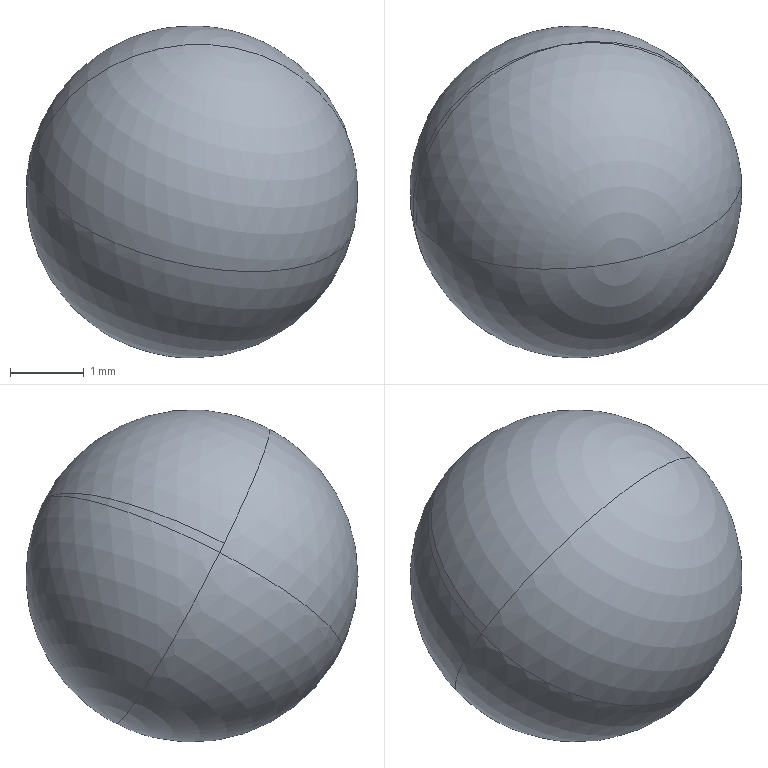Part | SolidWorks | features BaseBody 1 | 1 solid | 6 faces | box 4.5 x 4.5 x 4.5 mm | volume 47.713 mm3 | sphere 6
STEP:
#1=CARTESIAN_POINT('',(1921.673,-161.637,842.253));
#2=VERTEX_POINT('',#1);
#3=CARTESIAN_POINT('',(1924.058,-163.253,840.902));
#4=VERTEX_POINT('',#3);
#5=CARTESIAN_POINT('',(1921.862,-163.627,841.221));
#6=DIRECTION('',(-0.2015,0.436,-0.8771));
#7=DIRECTION('',(-0.08415,0.8844,0.459));
#8=AXIS2_PLACEMENT_3D('',#5,#6,#7);
#9=CIRCLE('',#8,2.25);
#10=EDGE_CURVE('',#2,#4,#9,.T.);
#11=ORIENTED_EDGE('',*,*,#10,.F.);
#12=CARTESIAN_POINT('',(1919.699,-164.062,841.662));
#13=VERTEX_POINT('',#12);
#14=CARTESIAN_POINT('',(1921.862,-163.627,841.221));
#15=DIRECTION('',(0.2623,-0.4247,0.8665));
#16=DIRECTION('',(0.,-0.8979,-0.4401));
#17=AXIS2_PLACEMENT_3D('',#14,#15,#16);
#18=CIRCLE('',#17,2.25);
#19=EDGE_CURVE('',#2,#13,#18,.T.);
#20=ORIENTED_EDGE('',*,*,#19,.T.);
#21=CARTESIAN_POINT('',(1921.862,-163.627,841.221));
#22=DIRECTION('',(-0.08415,0.8844,0.459));
#23=DIRECTION('',(0.2015,-0.436,0.8771));
#24=AXIS2_PLACEMENT_3D('',#21,#22,#23);
#25=CIRCLE('',#24,2.25);
#26=EDGE_CURVE('',#13,#4,#25,.T.);
#27=ORIENTED_EDGE('',*,*,#26,.T.);
#28=EDGE_LOOP('',(#11,#20,#27));
#29=FACE_OUTER_BOUND('',#28,.T.);
#30=CARTESIAN_POINT('',(1921.862,-163.627,841.221));
#31=DIRECTION('',(-0.2623,0.4247,-0.8665));
#32=DIRECTION('',(-0.9613,-0.1933,0.1963));
#33=AXIS2_PLACEMENT_3D('',#30,#31,#32);
#34=SPHERICAL_SURFACE('',#33,2.25);
#35=ADVANCED_FACE('',(#29),#34,.T.);
#36=CARTESIAN_POINT('',(1919.666,-164.001,841.539));
#37=VERTEX_POINT('',#36);
#38=CARTESIAN_POINT('',(1921.862,-163.627,841.221));
#39=DIRECTION('',(-0.2015,0.436,-0.8771));
#40=DIRECTION('',(-0.08415,0.8844,0.459));
#41=AXIS2_PLACEMENT_3D('',#38,#39,#40);
#42=CIRCLE('',#41,2.25);
#43=EDGE_CURVE('',#37,#2,#42,.T.);
#44=ORIENTED_EDGE('',*,*,#43,.T.);
#45=CARTESIAN_POINT('',(1924.025,-163.192,840.779));
#46=VERTEX_POINT('',#45);
#47=CARTESIAN_POINT('',(1921.862,-163.627,841.221));
#48=DIRECTION('',(-0.2623,0.4247,-0.8665));
#49=DIRECTION('',(0.,0.8979,0.4401));
#50=AXIS2_PLACEMENT_3D('',#47,#48,#49);
#51=CIRCLE('',#50,2.25);
#52=EDGE_CURVE('',#2,#46,#51,.T.);
#53=ORIENTED_EDGE('',*,*,#52,.T.);
#54=CARTESIAN_POINT('',(1921.862,-163.627,841.221));
#55=DIRECTION('',(0.08415,-0.8844,-0.459));
#56=DIRECTION('',(0.9759,0.1663,-0.1415));
#57=AXIS2_PLACEMENT_3D('',#54,#55,#56);
#58=CIRCLE('',#57,2.25);
#59=EDGE_CURVE('',#37,#46,#58,.T.);
#60=ORIENTED_EDGE('',*,*,#59,.F.);
#61=EDGE_LOOP('',(#44,#53,#60));
#62=FACE_OUTER_BOUND('',#61,.T.);
#63=CARTESIAN_POINT('',(1921.862,-163.627,841.221));
#64=DIRECTION('',(0.2623,-0.4247,0.8665));
#65=DIRECTION('',(0.9613,0.1933,-0.1963));
#66=AXIS2_PLACEMENT_3D('',#63,#64,#65);
#67=SPHERICAL_SURFACE('',#66,2.25);
#68=ADVANCED_FACE('',(#62),#67,.T.);
#69=ORIENTED_EDGE('',*,*,#59,.T.);
#70=CARTESIAN_POINT('',(1921.862,-163.627,841.221));
#71=DIRECTION('',(0.08415,-0.8844,-0.459));
#72=DIRECTION('',(0.9759,0.1663,-0.1415));
#73=AXIS2_PLACEMENT_3D('',#70,#71,#72);
#74=CIRCLE('',#73,2.25);
#75=EDGE_CURVE('',#46,#4,#74,.T.);
#76=ORIENTED_EDGE('',*,*,#75,.T.);
#77=CARTESIAN_POINT('',(1921.862,-163.627,841.221));
#78=DIRECTION('',(0.2015,-0.436,0.8771));
#79=DIRECTION('',(-0.9759,-0.1663,0.1415));
#80=AXIS2_PLACEMENT_3D('',#77,#78,#79);
#81=CIRCLE('',#80,2.25);
#82=EDGE_CURVE('',#37,#4,#81,.T.);
#83=ORIENTED_EDGE('',*,*,#82,.F.);
#84=EDGE_LOOP('',(#69,#76,#83));
#85=FACE_OUTER_BOUND('',#84,.T.);
#86=CARTESIAN_POINT('',(1921.862,-163.627,841.221));
#87=DIRECTION('',(-0.2623,0.4247,-0.8665));
#88=DIRECTION('',(-0.9613,-0.1933,0.1963));
#89=AXIS2_PLACEMENT_3D('',#86,#87,#88);
#90=SPHERICAL_SURFACE('',#89,2.25);
#91=ADVANCED_FACE('',(#85),#90,.T.);
#92=ORIENTED_EDGE('',*,*,#52,.F.);
#93=ORIENTED_EDGE('',*,*,#10,.T.);
#94=ORIENTED_EDGE('',*,*,#75,.F.);
#95=EDGE_LOOP('',(#92,#93,#94));
#96=FACE_OUTER_BOUND('',#95,.T.);
#97=CARTESIAN_POINT('',(1921.862,-163.627,841.221));
#98=DIRECTION('',(0.2623,-0.4247,0.8665));
#99=DIRECTION('',(0.9613,0.1933,-0.1963));
#100=AXIS2_PLACEMENT_3D('',#97,#98,#99);
#101=SPHERICAL_SURFACE('',#100,2.25);
#102=ADVANCED_FACE('',(#96),#101,.T.);
#103=ORIENTED_EDGE('',*,*,#19,.F.);
#104=ORIENTED_EDGE('',*,*,#43,.F.);
#105=CARTESIAN_POINT('',(1921.862,-163.627,841.221));
#106=DIRECTION('',(-0.08415,0.8844,0.459));
#107=DIRECTION('',(0.2015,-0.436,0.8771));
#108=AXIS2_PLACEMENT_3D('',#105,#106,#107);
#109=CIRCLE('',#108,2.25);
#110=EDGE_CURVE('',#37,#13,#109,.T.);
#111=ORIENTED_EDGE('',*,*,#110,.T.);
#112=EDGE_LOOP('',(#103,#104,#111));
#113=FACE_OUTER_BOUND('',#112,.T.);
#114=CARTESIAN_POINT('',(1921.862,-163.627,841.221));
#115=DIRECTION('',(-0.2623,0.4247,-0.8665));
#116=DIRECTION('',(-0.9613,-0.1933,0.1963));
#117=AXIS2_PLACEMENT_3D('',#114,#115,#116);
#118=SPHERICAL_SURFACE('',#117,2.25);
#119=ADVANCED_FACE('',(#113),#118,.T.);
#120=ORIENTED_EDGE('',*,*,#110,.F.);
#121=ORIENTED_EDGE('',*,*,#82,.T.);
#122=ORIENTED_EDGE('',*,*,#26,.F.);
#123=EDGE_LOOP('',(#120,#121,#122));
#124=FACE_OUTER_BOUND('',#123,.T.);
#125=CARTESIAN_POINT('',(1921.862,-163.627,841.221));
#126=DIRECTION('',(0.2623,-0.4247,0.8665));
#127=DIRECTION('',(0.9613,0.1933,-0.1963));
#128=AXIS2_PLACEMENT_3D('',#125,#126,#127);
#129=SPHERICAL_SURFACE('',#128,2.25);
#130=ADVANCED_FACE('',(#124),#129,.T.);
#131=CLOSED_SHELL('',(#35,#68,#91,#102,#119,#130));
#132=MANIFOLD_SOLID_BREP('',#131);
#133=CARTESIAN_POINT('',(0.,0.,0.));
#134=DIRECTION('',(0.,0.,1.));
#135=DIRECTION('',(1.,0.,0.));
#136=AXIS2_PLACEMENT_3D('',#133,#134,#135);
#137=(LENGTH_UNIT()NAMED_UNIT(*)SI_UNIT(.MILLI.,.METRE.));
#138=UNCERTAINTY_MEASURE_WITH_UNIT(LENGTH_MEASURE(0.00001),#137,'','');
#139=(NAMED_UNIT(*)PLANE_ANGLE_UNIT()SI_UNIT($,.RADIAN.));
#140=(NAMED_UNIT(*)SI_UNIT($,.STERADIAN.)SOLID_ANGLE_UNIT());
#141=(GEOMETRIC_REPRESENTATION_CONTEXT(3)GLOBAL_UNCERTAINTY_ASSIGNED_CONTEXT((#138))GLOBAL_UNIT_ASSIGNED_CONTEXT((#137,#139,#140))REPRESENTATION_CONTEXT('',''));
#142=ADVANCED_BREP_SHAPE_REPRESENTATION('',(#132,#136),#141);